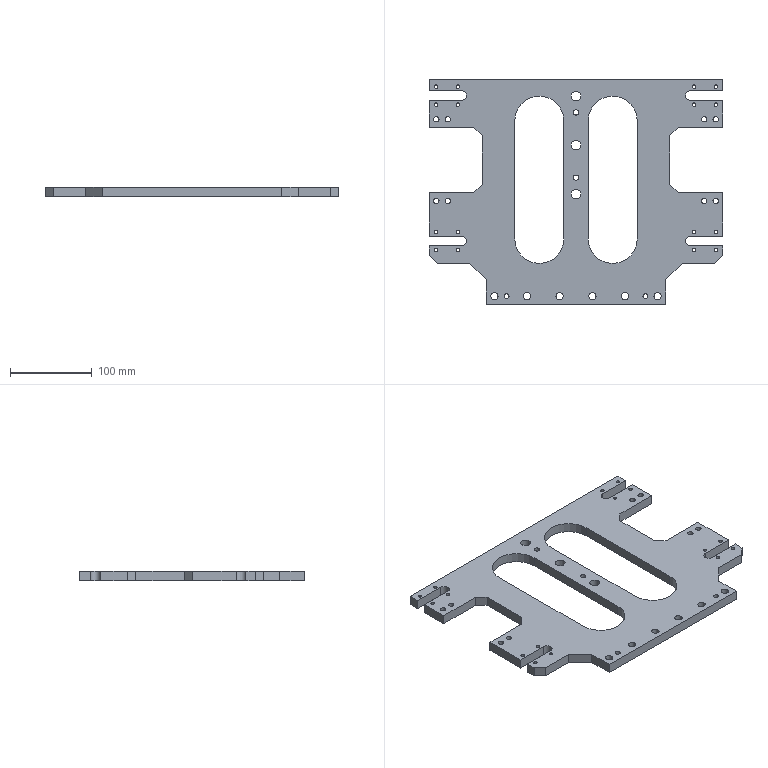CAM job | NX | 3-axis milling, drilling | part box 360 x 275 x 12 mm | stock box 364 x 279 x 12 mm
Tools:
number,name,description,diameter,corner_radius,flute_length,length,flutes
11,ZXZ,Milling Tool-5 Parameters,6.0,0.0,50.0,75.0,2
16,6.0ZT,Drilling Tool,6.0,0.0,35.0,50.0,2
17,6.6ZT,Drilling Tool,6.6,0.0,35.0,50.0,2
14,4.2ZT,Drilling Tool,4.2,0.0,35.0,50.0,2
19,9.0ZT,Drilling Tool,9.0,0.0,35.0,50.0,2
12,12.0ZT,Drilling Tool,11.0,0.0,35.0,50.0,2
10,D10,Milling Tool-5 Parameters,10.0,0.0,50.0,75.0,2
9,D10JING,Milling Tool-5 Parameters,10.0,0.0,50.0,75.0,2
6,D6,Milling Tool-5 Parameters,6.0,0.0,50.0,75.0,2
7,D6A45,Milling Tool-5 Parameters,6.0,0.0,3.0,3.0,2
Operations:
program,operation,operation_type,tool,method,geometry_group,spindle_rpm,surface_speed,feed_per_tooth,feed_cut,feed_plunge,cut_length_mm,path_length_mm,cut_time_min,machine_time_min
1压左右,DRILLING,Operation,ZXZ,METHOD,A,3000.0,56.0,0.0417,250.0,0.0,148.0,1845.446,0.592,0.7617
1压左右,DRILLING_COPY,Operation,6.0ZT,METHOD,A,2000.0,37.0,0.045,180.0,0.0,36.605,406.237,0.2034,0.2403
1压左右,DRILLING_COPY_COPY_2,Operation,6.6ZT,METHOD,A,2000.0,37.0,0.045,180.0,0.0,184.828,1210.927,1.027,1.129
1压左右,DRILLING_COPY_COPY_1,Operation,4.2ZT,METHOD,A,2000.0,37.0,0.045,180.0,0.0,284.189,1659.554,1.579,1.716
1压左右,DRILLING_COPY_COPY,Operation,9.0ZT,METHOD,A,1000.0,28.0,0.09,180.0,0.0,115.223,606.008,0.6401,0.6892
1压左右,DRILLING_COPY_COPY_COPY,Operation,12.0ZT,METHOD,A,1000.0,28.0,0.09,180.0,0.0,59.414,404.978,0.3301,0.3646
1压左右,ZLEVEL_PROFILE,ZLevelMilling,D10,METHOD,A,2200.0,69.0,0.5,2200.0,100.0,34946.648,35605.342,15.885,15.951
1压左右,ZLEVEL_PROFILE_COPY_1,ZLevelMilling,D10,METHOD,A,2200.0,69.0,0.5,2200.0,100.0,48297.357,48735.851,21.953,21.997
1压左右,ZLEVEL_PROFILE_COPY,ZLevelMilling,D10JING,METHOD,A,5000.0,157.0,0.12,1200.0,100.0,614.596,1272.786,0.5122,0.578
1压左右,ZLEVEL_PROFILE_COPY_COPY_1,ZLevelMilling,D6,METHOD,A,5000.0,157.0,0.12,1200.0,100.0,932.38,1492.252,0.777,0.833
1压左右,ZLEVEL_PROFILE_COPY_COPY,ZLevelMilling,D6A45,METHOD,A,7500.0,141.0,0.08,1200.0,100.0,2408.32,15880.464,2.007,3.354
2压前后,ZLEVEL_PROFILE_COPY_1_1,ZLevelMilling,D10,METHOD,A,2200.0,69.0,0.5,2200.0,100.0,71030.119,71625.67,32.286,32.346
2压前后,ZLEVEL_PROFILE_COPY_COPY_1_1,ZLevelMilling,D10JING,METHOD,A,5000.0,157.0,0.12,1200.0,100.0,1270.834,1865.804,1.059,1.119
2压前后,ZLEVEL_PROFILE_COPY_COPY_COPY,ZLevelMilling,D6A45,METHOD,A,7500.0,141.0,0.08,1200.0,100.0,1261.991,1937.82,1.052,1.119